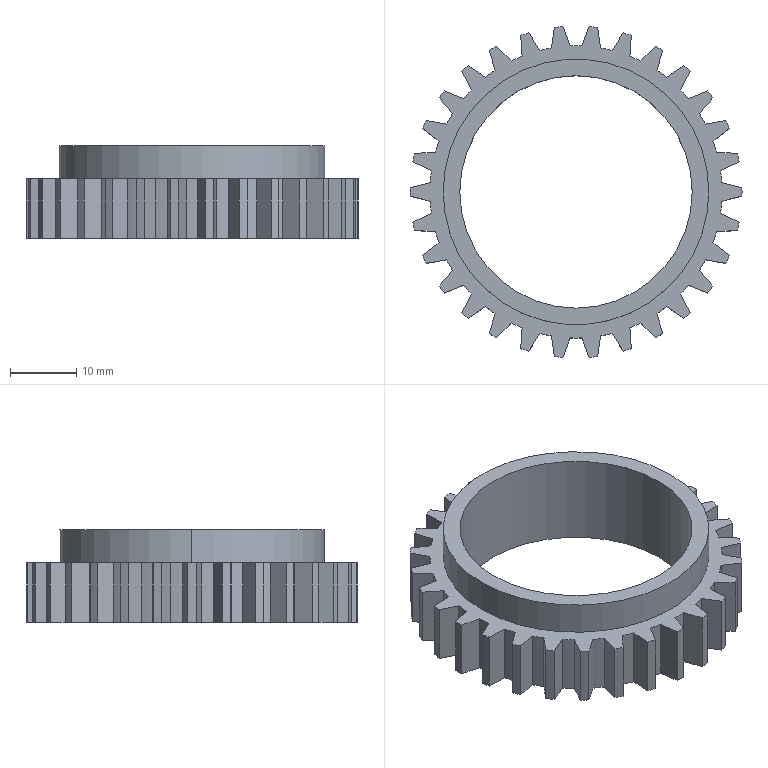Part | SolidWorks | features CirPattern 1, ICE 1, Revolution 1 | 1 solid | 128 faces | box 50 x 49.844 x 14 mm | volume 8157 mm3 | cylinder 65 | plane 63 | commonest cylinder face diameters 50 x31 44 x30 35 x2 40 x2